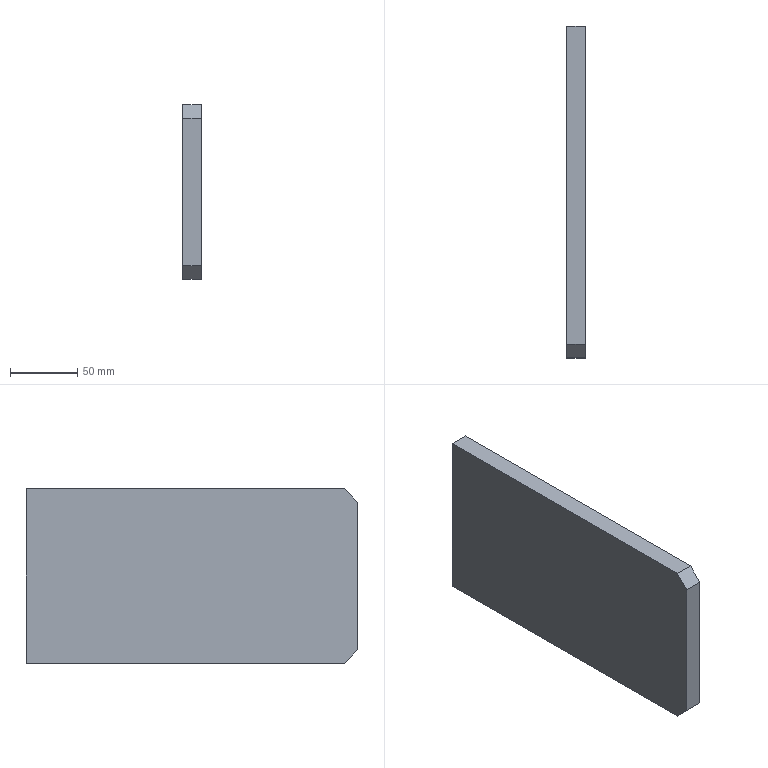Part | SolidWorks | features BaseBody 1 | 1 solid | 8 faces | box 14 x 247 x 130 mm | volume 448140 mm3 | plane 8
STEP:
#1=CARTESIAN_POINT('',(-7.,122.,65.));
#2=VERTEX_POINT('',#1);
#3=CARTESIAN_POINT('',(7.,122.,65.));
#4=VERTEX_POINT('',#3);
#5=CARTESIAN_POINT('',(7.,122.,65.));
#6=DIRECTION('',(1.,0.,0.));
#7=VECTOR('',#6,1000.);
#8=LINE('',#5,#7);
#9=EDGE_CURVE('',#2,#4,#8,.T.);
#10=ORIENTED_EDGE('',*,*,#9,.F.);
#11=CARTESIAN_POINT('',(-7.,-115.,65.));
#12=VERTEX_POINT('',#11);
#13=CARTESIAN_POINT('',(-7.,125.,65.));
#14=DIRECTION('',(0.,-1.,0.));
#15=VECTOR('',#14,1000.);
#16=LINE('',#13,#15);
#17=EDGE_CURVE('',#2,#12,#16,.T.);
#18=ORIENTED_EDGE('',*,*,#17,.T.);
#19=CARTESIAN_POINT('',(7.,-115.,65.));
#20=VERTEX_POINT('',#19);
#21=CARTESIAN_POINT('',(7.,-115.,65.));
#22=DIRECTION('',(-1.,0.,0.));
#23=VECTOR('',#22,1000.);
#24=LINE('',#21,#23);
#25=EDGE_CURVE('',#20,#12,#24,.T.);
#26=ORIENTED_EDGE('',*,*,#25,.F.);
#27=CARTESIAN_POINT('',(7.,125.,65.));
#28=DIRECTION('',(0.,-1.,0.));
#29=VECTOR('',#28,1000.);
#30=LINE('',#27,#29);
#31=EDGE_CURVE('',#4,#20,#30,.T.);
#32=ORIENTED_EDGE('',*,*,#31,.F.);
#33=EDGE_LOOP('',(#10,#18,#26,#32));
#34=FACE_OUTER_BOUND('',#33,.T.);
#35=CARTESIAN_POINT('',(7.,125.,65.));
#36=DIRECTION('',(0.,0.,-1.));
#37=DIRECTION('',(0.,1.,0.));
#38=AXIS2_PLACEMENT_3D('',#35,#36,#37);
#39=PLANE('',#38);
#40=ADVANCED_FACE('',(#34),#39,.F.);
#41=CARTESIAN_POINT('',(7.,122.,-65.));
#42=VERTEX_POINT('',#41);
#43=CARTESIAN_POINT('',(-7.,122.,-65.));
#44=VERTEX_POINT('',#43);
#45=CARTESIAN_POINT('',(7.,122.,-65.));
#46=DIRECTION('',(-1.,0.,0.));
#47=VECTOR('',#46,1000.);
#48=LINE('',#45,#47);
#49=EDGE_CURVE('',#42,#44,#48,.T.);
#50=ORIENTED_EDGE('',*,*,#49,.F.);
#51=CARTESIAN_POINT('',(7.,-115.,-65.));
#52=VERTEX_POINT('',#51);
#53=CARTESIAN_POINT('',(7.,125.,-65.));
#54=DIRECTION('',(0.,1.,0.));
#55=VECTOR('',#54,1000.);
#56=LINE('',#53,#55);
#57=EDGE_CURVE('',#52,#42,#56,.T.);
#58=ORIENTED_EDGE('',*,*,#57,.F.);
#59=CARTESIAN_POINT('',(-7.,-115.,-65.));
#60=VERTEX_POINT('',#59);
#61=CARTESIAN_POINT('',(7.,-115.,-65.));
#62=DIRECTION('',(-1.,0.,0.));
#63=VECTOR('',#62,1000.);
#64=LINE('',#61,#63);
#65=EDGE_CURVE('',#52,#60,#64,.T.);
#66=ORIENTED_EDGE('',*,*,#65,.T.);
#67=CARTESIAN_POINT('',(-7.,125.,-65.));
#68=DIRECTION('',(0.,1.,0.));
#69=VECTOR('',#68,1000.);
#70=LINE('',#67,#69);
#71=EDGE_CURVE('',#60,#44,#70,.T.);
#72=ORIENTED_EDGE('',*,*,#71,.T.);
#73=EDGE_LOOP('',(#50,#58,#66,#72));
#74=FACE_OUTER_BOUND('',#73,.T.);
#75=CARTESIAN_POINT('',(7.,125.,-65.));
#76=DIRECTION('',(0.,0.,1.));
#77=DIRECTION('',(0.,-1.,0.));
#78=AXIS2_PLACEMENT_3D('',#75,#76,#77);
#79=PLANE('',#78);
#80=ADVANCED_FACE('',(#74),#79,.F.);
#81=ORIENTED_EDGE('',*,*,#57,.T.);
#82=CARTESIAN_POINT('',(7.,122.,0.));
#83=DIRECTION('',(0.,0.,1.));
#84=VECTOR('',#83,1000.);
#85=LINE('',#82,#84);
#86=EDGE_CURVE('',#42,#4,#85,.T.);
#87=ORIENTED_EDGE('',*,*,#86,.T.);
#88=ORIENTED_EDGE('',*,*,#31,.T.);
#89=CARTESIAN_POINT('',(7.,-125.,55.));
#90=VERTEX_POINT('',#89);
#91=CARTESIAN_POINT('',(7.,-115.,65.));
#92=DIRECTION('',(0.,-0.7071,-0.7071));
#93=VECTOR('',#92,1000.);
#94=LINE('',#91,#93);
#95=EDGE_CURVE('',#20,#90,#94,.T.);
#96=ORIENTED_EDGE('',*,*,#95,.T.);
#97=CARTESIAN_POINT('',(7.,-125.,-55.));
#98=VERTEX_POINT('',#97);
#99=CARTESIAN_POINT('',(7.,-125.,55.));
#100=DIRECTION('',(0.,0.,-1.));
#101=VECTOR('',#100,1000.);
#102=LINE('',#99,#101);
#103=EDGE_CURVE('',#90,#98,#102,.T.);
#104=ORIENTED_EDGE('',*,*,#103,.T.);
#105=CARTESIAN_POINT('',(7.,-125.,-55.));
#106=DIRECTION('',(0.,0.7071,-0.7071));
#107=VECTOR('',#106,1000.);
#108=LINE('',#105,#107);
#109=EDGE_CURVE('',#98,#52,#108,.T.);
#110=ORIENTED_EDGE('',*,*,#109,.T.);
#111=EDGE_LOOP('',(#81,#87,#88,#96,#104,#110));
#112=FACE_OUTER_BOUND('',#111,.T.);
#113=CARTESIAN_POINT('',(7.,0.,0.));
#114=DIRECTION('',(1.,0.,0.));
#115=DIRECTION('',(0.,0.,-1.));
#116=AXIS2_PLACEMENT_3D('',#113,#114,#115);
#117=PLANE('',#116);
#118=ADVANCED_FACE('',(#112),#117,.T.);
#119=CARTESIAN_POINT('',(-7.,122.,0.));
#120=DIRECTION('',(0.,0.,1.));
#121=VECTOR('',#120,1000.);
#122=LINE('',#119,#121);
#123=EDGE_CURVE('',#44,#2,#122,.T.);
#124=ORIENTED_EDGE('',*,*,#123,.F.);
#125=ORIENTED_EDGE('',*,*,#71,.F.);
#126=CARTESIAN_POINT('',(-7.,-125.,-55.));
#127=VERTEX_POINT('',#126);
#128=CARTESIAN_POINT('',(-7.,-125.,-55.));
#129=DIRECTION('',(0.,0.7071,-0.7071));
#130=VECTOR('',#129,1000.);
#131=LINE('',#128,#130);
#132=EDGE_CURVE('',#127,#60,#131,.T.);
#133=ORIENTED_EDGE('',*,*,#132,.F.);
#134=CARTESIAN_POINT('',(-7.,-125.,55.));
#135=VERTEX_POINT('',#134);
#136=CARTESIAN_POINT('',(-7.,-125.,55.));
#137=DIRECTION('',(0.,0.,-1.));
#138=VECTOR('',#137,1000.);
#139=LINE('',#136,#138);
#140=EDGE_CURVE('',#135,#127,#139,.T.);
#141=ORIENTED_EDGE('',*,*,#140,.F.);
#142=CARTESIAN_POINT('',(-7.,-115.,65.));
#143=DIRECTION('',(0.,-0.7071,-0.7071));
#144=VECTOR('',#143,1000.);
#145=LINE('',#142,#144);
#146=EDGE_CURVE('',#12,#135,#145,.T.);
#147=ORIENTED_EDGE('',*,*,#146,.F.);
#148=ORIENTED_EDGE('',*,*,#17,.F.);
#149=EDGE_LOOP('',(#124,#125,#133,#141,#147,#148));
#150=FACE_OUTER_BOUND('',#149,.T.);
#151=CARTESIAN_POINT('',(-7.,0.,0.));
#152=DIRECTION('',(1.,0.,0.));
#153=DIRECTION('',(0.,0.,-1.));
#154=AXIS2_PLACEMENT_3D('',#151,#152,#153);
#155=PLANE('',#154);
#156=ADVANCED_FACE('',(#150),#155,.F.);
#157=ORIENTED_EDGE('',*,*,#146,.T.);
#158=CARTESIAN_POINT('',(7.,-125.,55.));
#159=DIRECTION('',(-1.,0.,0.));
#160=VECTOR('',#159,1000.);
#161=LINE('',#158,#160);
#162=EDGE_CURVE('',#90,#135,#161,.T.);
#163=ORIENTED_EDGE('',*,*,#162,.F.);
#164=ORIENTED_EDGE('',*,*,#95,.F.);
#165=ORIENTED_EDGE('',*,*,#25,.T.);
#166=EDGE_LOOP('',(#157,#163,#164,#165));
#167=FACE_OUTER_BOUND('',#166,.T.);
#168=CARTESIAN_POINT('',(7.,-115.,65.));
#169=DIRECTION('',(0.,0.7071,-0.7071));
#170=DIRECTION('',(0.,0.7071,0.7071));
#171=AXIS2_PLACEMENT_3D('',#168,#169,#170);
#172=PLANE('',#171);
#173=ADVANCED_FACE('',(#167),#172,.F.);
#174=ORIENTED_EDGE('',*,*,#140,.T.);
#175=CARTESIAN_POINT('',(7.,-125.,-55.));
#176=DIRECTION('',(-1.,0.,0.));
#177=VECTOR('',#176,1000.);
#178=LINE('',#175,#177);
#179=EDGE_CURVE('',#98,#127,#178,.T.);
#180=ORIENTED_EDGE('',*,*,#179,.F.);
#181=ORIENTED_EDGE('',*,*,#103,.F.);
#182=ORIENTED_EDGE('',*,*,#162,.T.);
#183=EDGE_LOOP('',(#174,#180,#181,#182));
#184=FACE_OUTER_BOUND('',#183,.T.);
#185=CARTESIAN_POINT('',(7.,-125.,55.));
#186=DIRECTION('',(0.,1.,0.));
#187=DIRECTION('',(0.,0.,1.));
#188=AXIS2_PLACEMENT_3D('',#185,#186,#187);
#189=PLANE('',#188);
#190=ADVANCED_FACE('',(#184),#189,.F.);
#191=ORIENTED_EDGE('',*,*,#132,.T.);
#192=ORIENTED_EDGE('',*,*,#65,.F.);
#193=ORIENTED_EDGE('',*,*,#109,.F.);
#194=ORIENTED_EDGE('',*,*,#179,.T.);
#195=EDGE_LOOP('',(#191,#192,#193,#194));
#196=FACE_OUTER_BOUND('',#195,.T.);
#197=CARTESIAN_POINT('',(7.,-125.,-55.));
#198=DIRECTION('',(0.,0.7071,0.7071));
#199=DIRECTION('',(0.,-0.7071,0.7071));
#200=AXIS2_PLACEMENT_3D('',#197,#198,#199);
#201=PLANE('',#200);
#202=ADVANCED_FACE('',(#196),#201,.F.);
#203=ORIENTED_EDGE('',*,*,#9,.T.);
#204=ORIENTED_EDGE('',*,*,#86,.F.);
#205=ORIENTED_EDGE('',*,*,#49,.T.);
#206=ORIENTED_EDGE('',*,*,#123,.T.);
#207=EDGE_LOOP('',(#203,#204,#205,#206));
#208=FACE_OUTER_BOUND('',#207,.T.);
#209=CARTESIAN_POINT('',(-587.,122.,0.));
#210=DIRECTION('',(0.,1.,0.));
#211=DIRECTION('',(0.,0.,-1.));
#212=AXIS2_PLACEMENT_3D('',#209,#210,#211);
#213=PLANE('',#212);
#214=ADVANCED_FACE('',(#208),#213,.T.);
#215=CLOSED_SHELL('',(#40,#80,#118,#156,#173,#190,#202,#214));
#216=MANIFOLD_SOLID_BREP('',#215);
#217=CARTESIAN_POINT('',(0.,0.,0.));
#218=DIRECTION('',(0.,0.,1.));
#219=DIRECTION('',(1.,0.,0.));
#220=AXIS2_PLACEMENT_3D('',#217,#218,#219);
#221=(LENGTH_UNIT()NAMED_UNIT(*)SI_UNIT(.MILLI.,.METRE.));
#222=UNCERTAINTY_MEASURE_WITH_UNIT(LENGTH_MEASURE(0.00001),#221,'','');
#223=(NAMED_UNIT(*)PLANE_ANGLE_UNIT()SI_UNIT($,.RADIAN.));
#224=(NAMED_UNIT(*)SI_UNIT($,.STERADIAN.)SOLID_ANGLE_UNIT());
#225=(GEOMETRIC_REPRESENTATION_CONTEXT(3)GLOBAL_UNCERTAINTY_ASSIGNED_CONTEXT((#222))GLOBAL_UNIT_ASSIGNED_CONTEXT((#221,#223,#224))REPRESENTATION_CONTEXT('',''));
#226=ADVANCED_BREP_SHAPE_REPRESENTATION('',(#216,#220),#225);